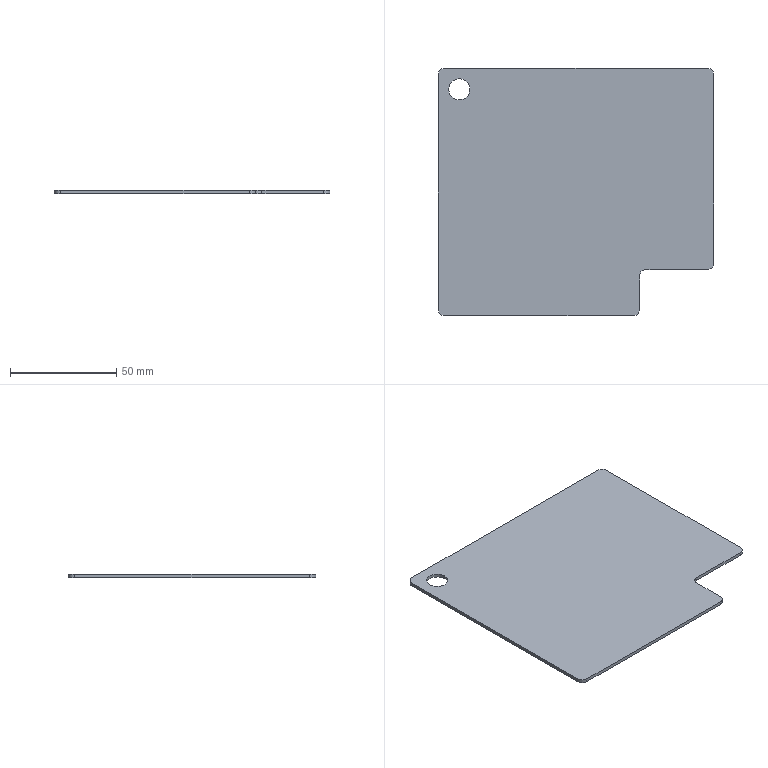Part | SolidWorks | features FlatPattern 1, SMBaseFlange 1, SheetMetal 1 | 1 solid | 16 faces | box 130 x 116.815 x 1.6 mm | volume 22938 mm3 | cylinder 8 | plane 8 | commonest cylinder face diameters 6 x6 10 x2
STEP:
#1=CARTESIAN_POINT('',(5.,272.5,1.6));
#2=VERTEX_POINT('',#1);
#3=CARTESIAN_POINT('',(15.,272.5,1.6));
#4=VERTEX_POINT('',#3);
#5=CARTESIAN_POINT('',(10.,272.5,1.6));
#6=DIRECTION('',(0.,0.,1.));
#7=DIRECTION('',(1.,0.,0.));
#8=AXIS2_PLACEMENT_3D('',#5,#6,#7);
#9=CIRCLE('',#8,5.);
#10=EDGE_CURVE('',#2,#4,#9,.T.);
#11=ORIENTED_EDGE('',*,*,#10,.T.);
#12=CARTESIAN_POINT('',(15.,272.5,0.));
#13=VERTEX_POINT('',#12);
#14=CARTESIAN_POINT('',(15.,272.5,1.6));
#15=DIRECTION('',(0.,0.,-1.));
#16=VECTOR('',#15,1000.);
#17=LINE('',#14,#16);
#18=EDGE_CURVE('',#4,#13,#17,.T.);
#19=ORIENTED_EDGE('',*,*,#18,.T.);
#20=CARTESIAN_POINT('',(5.,272.5,0.));
#21=VERTEX_POINT('',#20);
#22=CARTESIAN_POINT('',(10.,272.5,0.));
#23=DIRECTION('',(0.,0.,1.));
#24=DIRECTION('',(1.,0.,0.));
#25=AXIS2_PLACEMENT_3D('',#22,#23,#24);
#26=CIRCLE('',#25,5.);
#27=EDGE_CURVE('',#21,#13,#26,.T.);
#28=ORIENTED_EDGE('',*,*,#27,.F.);
#29=CARTESIAN_POINT('',(5.,272.5,1.6));
#30=DIRECTION('',(0.,0.,-1.));
#31=VECTOR('',#30,1000.);
#32=LINE('',#29,#31);
#33=EDGE_CURVE('',#2,#21,#32,.T.);
#34=ORIENTED_EDGE('',*,*,#33,.F.);
#35=EDGE_LOOP('',(#11,#19,#28,#34));
#36=FACE_OUTER_BOUND('',#35,.T.);
#37=CARTESIAN_POINT('',(10.,272.5,1.6));
#38=DIRECTION('',(0.,0.,-1.));
#39=DIRECTION('',(-1.,0.,0.));
#40=AXIS2_PLACEMENT_3D('',#37,#38,#39);
#41=CYLINDRICAL_SURFACE('',#40,5.);
#42=ADVANCED_FACE('',(#36),#41,.F.);
#43=CARTESIAN_POINT('',(0.,168.685,1.6));
#44=VERTEX_POINT('',#43);
#45=CARTESIAN_POINT('',(3.,165.685,1.6));
#46=VERTEX_POINT('',#45);
#47=CARTESIAN_POINT('',(3.,168.685,1.6));
#48=DIRECTION('',(0.,0.,1.));
#49=DIRECTION('',(-1.,0.,0.));
#50=AXIS2_PLACEMENT_3D('',#47,#48,#49);
#51=CIRCLE('',#50,3.);
#52=EDGE_CURVE('',#44,#46,#51,.T.);
#53=ORIENTED_EDGE('',*,*,#52,.T.);
#54=CARTESIAN_POINT('',(92.,165.685,1.6));
#55=VERTEX_POINT('',#54);
#56=CARTESIAN_POINT('',(92.,165.685,1.6));
#57=DIRECTION('',(1.,0.,0.));
#58=VECTOR('',#57,1000.);
#59=LINE('',#56,#58);
#60=EDGE_CURVE('',#46,#55,#59,.T.);
#61=ORIENTED_EDGE('',*,*,#60,.T.);
#62=CARTESIAN_POINT('',(95.,168.685,1.6));
#63=VERTEX_POINT('',#62);
#64=CARTESIAN_POINT('',(92.,168.685,1.6));
#65=DIRECTION('',(0.,0.,1.));
#66=DIRECTION('',(-1.,0.,0.));
#67=AXIS2_PLACEMENT_3D('',#64,#65,#66);
#68=CIRCLE('',#67,3.);
#69=EDGE_CURVE('',#55,#63,#68,.T.);
#70=ORIENTED_EDGE('',*,*,#69,.T.);
#71=CARTESIAN_POINT('',(95.,184.5,1.6));
#72=VERTEX_POINT('',#71);
#73=CARTESIAN_POINT('',(95.,184.5,1.6));
#74=DIRECTION('',(0.,1.,0.));
#75=VECTOR('',#74,1000.);
#76=LINE('',#73,#75);
#77=EDGE_CURVE('',#63,#72,#76,.T.);
#78=ORIENTED_EDGE('',*,*,#77,.T.);
#79=CARTESIAN_POINT('',(98.,187.5,1.6));
#80=VERTEX_POINT('',#79);
#81=CARTESIAN_POINT('',(98.,184.5,1.6));
#82=DIRECTION('',(0.,0.,-1.));
#83=DIRECTION('',(1.,0.,0.));
#84=AXIS2_PLACEMENT_3D('',#81,#82,#83);
#85=CIRCLE('',#84,3.);
#86=EDGE_CURVE('',#72,#80,#85,.T.);
#87=ORIENTED_EDGE('',*,*,#86,.T.);
#88=CARTESIAN_POINT('',(127.,187.5,1.6));
#89=VERTEX_POINT('',#88);
#90=CARTESIAN_POINT('',(127.,187.5,1.6));
#91=DIRECTION('',(1.,0.,0.));
#92=VECTOR('',#91,1000.);
#93=LINE('',#90,#92);
#94=EDGE_CURVE('',#80,#89,#93,.T.);
#95=ORIENTED_EDGE('',*,*,#94,.T.);
#96=CARTESIAN_POINT('',(130.,190.5,1.6));
#97=VERTEX_POINT('',#96);
#98=CARTESIAN_POINT('',(127.,190.5,1.6));
#99=DIRECTION('',(0.,0.,1.));
#100=DIRECTION('',(-1.,0.,0.));
#101=AXIS2_PLACEMENT_3D('',#98,#99,#100);
#102=CIRCLE('',#101,3.);
#103=EDGE_CURVE('',#89,#97,#102,.T.);
#104=ORIENTED_EDGE('',*,*,#103,.T.);
#105=CARTESIAN_POINT('',(130.,279.5,1.6));
#106=VERTEX_POINT('',#105);
#107=CARTESIAN_POINT('',(130.,279.5,1.6));
#108=DIRECTION('',(0.,1.,0.));
#109=VECTOR('',#108,1000.);
#110=LINE('',#107,#109);
#111=EDGE_CURVE('',#97,#106,#110,.T.);
#112=ORIENTED_EDGE('',*,*,#111,.T.);
#113=CARTESIAN_POINT('',(127.,282.5,1.6));
#114=VERTEX_POINT('',#113);
#115=CARTESIAN_POINT('',(127.,279.5,1.6));
#116=DIRECTION('',(0.,0.,1.));
#117=DIRECTION('',(-1.,0.,0.));
#118=AXIS2_PLACEMENT_3D('',#115,#116,#117);
#119=CIRCLE('',#118,3.);
#120=EDGE_CURVE('',#106,#114,#119,.T.);
#121=ORIENTED_EDGE('',*,*,#120,.T.);
#122=CARTESIAN_POINT('',(3.,282.5,1.6));
#123=VERTEX_POINT('',#122);
#124=CARTESIAN_POINT('',(3.,282.5,1.6));
#125=DIRECTION('',(-1.,0.,0.));
#126=VECTOR('',#125,1000.);
#127=LINE('',#124,#126);
#128=EDGE_CURVE('',#114,#123,#127,.T.);
#129=ORIENTED_EDGE('',*,*,#128,.T.);
#130=CARTESIAN_POINT('',(0.,279.5,1.6));
#131=VERTEX_POINT('',#130);
#132=CARTESIAN_POINT('',(3.,279.5,1.6));
#133=DIRECTION('',(0.,0.,1.));
#134=DIRECTION('',(1.,0.,0.));
#135=AXIS2_PLACEMENT_3D('',#132,#133,#134);
#136=CIRCLE('',#135,3.);
#137=EDGE_CURVE('',#123,#131,#136,.T.);
#138=ORIENTED_EDGE('',*,*,#137,.T.);
#139=CARTESIAN_POINT('',(0.,168.685,1.6));
#140=DIRECTION('',(0.,-1.,0.));
#141=VECTOR('',#140,1000.);
#142=LINE('',#139,#141);
#143=EDGE_CURVE('',#131,#44,#142,.T.);
#144=ORIENTED_EDGE('',*,*,#143,.T.);
#145=EDGE_LOOP('',(#53,#61,#70,#78,#87,#95,#104,#112,#121,#129,#138,#144));
#146=FACE_OUTER_BOUND('',#145,.T.);
#147=ORIENTED_EDGE('',*,*,#10,.F.);
#148=CARTESIAN_POINT('',(10.,272.5,1.6));
#149=DIRECTION('',(0.,0.,1.));
#150=DIRECTION('',(1.,0.,0.));
#151=AXIS2_PLACEMENT_3D('',#148,#149,#150);
#152=CIRCLE('',#151,5.);
#153=EDGE_CURVE('',#4,#2,#152,.T.);
#154=ORIENTED_EDGE('',*,*,#153,.F.);
#155=EDGE_LOOP('',(#147,#154));
#156=FACE_BOUND('',#155,.T.);
#157=CARTESIAN_POINT('',(3.,168.685,1.6));
#158=DIRECTION('',(0.,0.,-1.));
#159=DIRECTION('',(-1.,0.,0.));
#160=AXIS2_PLACEMENT_3D('',#157,#158,#159);
#161=PLANE('',#160);
#162=ADVANCED_FACE('',(#146,#156),#161,.F.);
#163=CARTESIAN_POINT('',(0.,168.685,0.));
#164=VERTEX_POINT('',#163);
#165=CARTESIAN_POINT('',(3.,165.685,0.));
#166=VERTEX_POINT('',#165);
#167=CARTESIAN_POINT('',(3.,168.685,0.));
#168=DIRECTION('',(0.,0.,1.));
#169=DIRECTION('',(-1.,0.,0.));
#170=AXIS2_PLACEMENT_3D('',#167,#168,#169);
#171=CIRCLE('',#170,3.);
#172=EDGE_CURVE('',#164,#166,#171,.T.);
#173=ORIENTED_EDGE('',*,*,#172,.F.);
#174=CARTESIAN_POINT('',(0.,279.5,0.));
#175=VERTEX_POINT('',#174);
#176=CARTESIAN_POINT('',(0.,168.685,0.));
#177=DIRECTION('',(0.,-1.,0.));
#178=VECTOR('',#177,1000.);
#179=LINE('',#176,#178);
#180=EDGE_CURVE('',#175,#164,#179,.T.);
#181=ORIENTED_EDGE('',*,*,#180,.F.);
#182=CARTESIAN_POINT('',(3.,282.5,0.));
#183=VERTEX_POINT('',#182);
#184=CARTESIAN_POINT('',(3.,279.5,0.));
#185=DIRECTION('',(0.,0.,1.));
#186=DIRECTION('',(1.,0.,0.));
#187=AXIS2_PLACEMENT_3D('',#184,#185,#186);
#188=CIRCLE('',#187,3.);
#189=EDGE_CURVE('',#183,#175,#188,.T.);
#190=ORIENTED_EDGE('',*,*,#189,.F.);
#191=CARTESIAN_POINT('',(127.,282.5,0.));
#192=VERTEX_POINT('',#191);
#193=CARTESIAN_POINT('',(3.,282.5,0.));
#194=DIRECTION('',(-1.,0.,0.));
#195=VECTOR('',#194,1000.);
#196=LINE('',#193,#195);
#197=EDGE_CURVE('',#192,#183,#196,.T.);
#198=ORIENTED_EDGE('',*,*,#197,.F.);
#199=CARTESIAN_POINT('',(130.,279.5,0.));
#200=VERTEX_POINT('',#199);
#201=CARTESIAN_POINT('',(127.,279.5,0.));
#202=DIRECTION('',(0.,0.,1.));
#203=DIRECTION('',(-1.,0.,0.));
#204=AXIS2_PLACEMENT_3D('',#201,#202,#203);
#205=CIRCLE('',#204,3.);
#206=EDGE_CURVE('',#200,#192,#205,.T.);
#207=ORIENTED_EDGE('',*,*,#206,.F.);
#208=CARTESIAN_POINT('',(130.,190.5,0.));
#209=VERTEX_POINT('',#208);
#210=CARTESIAN_POINT('',(130.,279.5,0.));
#211=DIRECTION('',(0.,1.,0.));
#212=VECTOR('',#211,1000.);
#213=LINE('',#210,#212);
#214=EDGE_CURVE('',#209,#200,#213,.T.);
#215=ORIENTED_EDGE('',*,*,#214,.F.);
#216=CARTESIAN_POINT('',(127.,187.5,0.));
#217=VERTEX_POINT('',#216);
#218=CARTESIAN_POINT('',(127.,190.5,0.));
#219=DIRECTION('',(0.,0.,1.));
#220=DIRECTION('',(-1.,0.,0.));
#221=AXIS2_PLACEMENT_3D('',#218,#219,#220);
#222=CIRCLE('',#221,3.);
#223=EDGE_CURVE('',#217,#209,#222,.T.);
#224=ORIENTED_EDGE('',*,*,#223,.F.);
#225=CARTESIAN_POINT('',(98.,187.5,0.));
#226=VERTEX_POINT('',#225);
#227=CARTESIAN_POINT('',(127.,187.5,0.));
#228=DIRECTION('',(1.,0.,0.));
#229=VECTOR('',#228,1000.);
#230=LINE('',#227,#229);
#231=EDGE_CURVE('',#226,#217,#230,.T.);
#232=ORIENTED_EDGE('',*,*,#231,.F.);
#233=CARTESIAN_POINT('',(95.,184.5,0.));
#234=VERTEX_POINT('',#233);
#235=CARTESIAN_POINT('',(98.,184.5,0.));
#236=DIRECTION('',(0.,0.,-1.));
#237=DIRECTION('',(1.,0.,0.));
#238=AXIS2_PLACEMENT_3D('',#235,#236,#237);
#239=CIRCLE('',#238,3.);
#240=EDGE_CURVE('',#234,#226,#239,.T.);
#241=ORIENTED_EDGE('',*,*,#240,.F.);
#242=CARTESIAN_POINT('',(95.,168.685,0.));
#243=VERTEX_POINT('',#242);
#244=CARTESIAN_POINT('',(95.,184.5,0.));
#245=DIRECTION('',(0.,1.,0.));
#246=VECTOR('',#245,1000.);
#247=LINE('',#244,#246);
#248=EDGE_CURVE('',#243,#234,#247,.T.);
#249=ORIENTED_EDGE('',*,*,#248,.F.);
#250=CARTESIAN_POINT('',(92.,165.685,0.));
#251=VERTEX_POINT('',#250);
#252=CARTESIAN_POINT('',(92.,168.685,0.));
#253=DIRECTION('',(0.,0.,1.));
#254=DIRECTION('',(-1.,0.,0.));
#255=AXIS2_PLACEMENT_3D('',#252,#253,#254);
#256=CIRCLE('',#255,3.);
#257=EDGE_CURVE('',#251,#243,#256,.T.);
#258=ORIENTED_EDGE('',*,*,#257,.F.);
#259=CARTESIAN_POINT('',(92.,165.685,0.));
#260=DIRECTION('',(1.,0.,0.));
#261=VECTOR('',#260,1000.);
#262=LINE('',#259,#261);
#263=EDGE_CURVE('',#166,#251,#262,.T.);
#264=ORIENTED_EDGE('',*,*,#263,.F.);
#265=EDGE_LOOP('',(#173,#181,#190,#198,#207,#215,#224,#232,#241,#249,#258,#264));
#266=FACE_OUTER_BOUND('',#265,.T.);
#267=ORIENTED_EDGE('',*,*,#27,.T.);
#268=CARTESIAN_POINT('',(10.,272.5,0.));
#269=DIRECTION('',(0.,0.,1.));
#270=DIRECTION('',(1.,0.,0.));
#271=AXIS2_PLACEMENT_3D('',#268,#269,#270);
#272=CIRCLE('',#271,5.);
#273=EDGE_CURVE('',#13,#21,#272,.T.);
#274=ORIENTED_EDGE('',*,*,#273,.T.);
#275=EDGE_LOOP('',(#267,#274));
#276=FACE_BOUND('',#275,.T.);
#277=CARTESIAN_POINT('',(3.,168.685,0.));
#278=DIRECTION('',(0.,0.,-1.));
#279=DIRECTION('',(-1.,0.,0.));
#280=AXIS2_PLACEMENT_3D('',#277,#278,#279);
#281=PLANE('',#280);
#282=ADVANCED_FACE('',(#266,#276),#281,.T.);
#283=ORIENTED_EDGE('',*,*,#172,.T.);
#284=CARTESIAN_POINT('',(3.,165.685,1.6));
#285=DIRECTION('',(0.,0.,-1.));
#286=VECTOR('',#285,1000.);
#287=LINE('',#284,#286);
#288=EDGE_CURVE('',#46,#166,#287,.T.);
#289=ORIENTED_EDGE('',*,*,#288,.F.);
#290=ORIENTED_EDGE('',*,*,#52,.F.);
#291=CARTESIAN_POINT('',(0.,168.685,1.6));
#292=DIRECTION('',(0.,0.,-1.));
#293=VECTOR('',#292,1000.);
#294=LINE('',#291,#293);
#295=EDGE_CURVE('',#44,#164,#294,.T.);
#296=ORIENTED_EDGE('',*,*,#295,.T.);
#297=EDGE_LOOP('',(#283,#289,#290,#296));
#298=FACE_OUTER_BOUND('',#297,.T.);
#299=CARTESIAN_POINT('',(3.,168.685,1.6));
#300=DIRECTION('',(0.,0.,-1.));
#301=DIRECTION('',(-1.,0.,0.));
#302=AXIS2_PLACEMENT_3D('',#299,#300,#301);
#303=CYLINDRICAL_SURFACE('',#302,3.);
#304=ADVANCED_FACE('',(#298),#303,.T.);
#305=ORIENTED_EDGE('',*,*,#263,.T.);
#306=CARTESIAN_POINT('',(92.,165.685,1.6));
#307=DIRECTION('',(0.,0.,-1.));
#308=VECTOR('',#307,1000.);
#309=LINE('',#306,#308);
#310=EDGE_CURVE('',#55,#251,#309,.T.);
#311=ORIENTED_EDGE('',*,*,#310,.F.);
#312=ORIENTED_EDGE('',*,*,#60,.F.);
#313=ORIENTED_EDGE('',*,*,#288,.T.);
#314=EDGE_LOOP('',(#305,#311,#312,#313));
#315=FACE_OUTER_BOUND('',#314,.T.);
#316=CARTESIAN_POINT('',(92.,165.685,1.6));
#317=DIRECTION('',(0.,1.,0.));
#318=DIRECTION('',(0.,0.,1.));
#319=AXIS2_PLACEMENT_3D('',#316,#317,#318);
#320=PLANE('',#319);
#321=ADVANCED_FACE('',(#315),#320,.F.);
#322=ORIENTED_EDGE('',*,*,#257,.T.);
#323=CARTESIAN_POINT('',(95.,168.685,1.6));
#324=DIRECTION('',(0.,0.,-1.));
#325=VECTOR('',#324,1000.);
#326=LINE('',#323,#325);
#327=EDGE_CURVE('',#63,#243,#326,.T.);
#328=ORIENTED_EDGE('',*,*,#327,.F.);
#329=ORIENTED_EDGE('',*,*,#69,.F.);
#330=ORIENTED_EDGE('',*,*,#310,.T.);
#331=EDGE_LOOP('',(#322,#328,#329,#330));
#332=FACE_OUTER_BOUND('',#331,.T.);
#333=CARTESIAN_POINT('',(92.,168.685,1.6));
#334=DIRECTION('',(0.,0.,-1.));
#335=DIRECTION('',(-1.,0.,0.));
#336=AXIS2_PLACEMENT_3D('',#333,#334,#335);
#337=CYLINDRICAL_SURFACE('',#336,3.);
#338=ADVANCED_FACE('',(#332),#337,.T.);
#339=ORIENTED_EDGE('',*,*,#248,.T.);
#340=CARTESIAN_POINT('',(95.,184.5,1.6));
#341=DIRECTION('',(0.,0.,-1.));
#342=VECTOR('',#341,1000.);
#343=LINE('',#340,#342);
#344=EDGE_CURVE('',#72,#234,#343,.T.);
#345=ORIENTED_EDGE('',*,*,#344,.F.);
#346=ORIENTED_EDGE('',*,*,#77,.F.);
#347=ORIENTED_EDGE('',*,*,#327,.T.);
#348=EDGE_LOOP('',(#339,#345,#346,#347));
#349=FACE_OUTER_BOUND('',#348,.T.);
#350=CARTESIAN_POINT('',(95.,184.5,1.6));
#351=DIRECTION('',(-1.,0.,0.));
#352=DIRECTION('',(0.,0.,1.));
#353=AXIS2_PLACEMENT_3D('',#350,#351,#352);
#354=PLANE('',#353);
#355=ADVANCED_FACE('',(#349),#354,.F.);
#356=ORIENTED_EDGE('',*,*,#240,.T.);
#357=CARTESIAN_POINT('',(98.,187.5,1.6));
#358=DIRECTION('',(0.,0.,-1.));
#359=VECTOR('',#358,1000.);
#360=LINE('',#357,#359);
#361=EDGE_CURVE('',#80,#226,#360,.T.);
#362=ORIENTED_EDGE('',*,*,#361,.F.);
#363=ORIENTED_EDGE('',*,*,#86,.F.);
#364=ORIENTED_EDGE('',*,*,#344,.T.);
#365=EDGE_LOOP('',(#356,#362,#363,#364));
#366=FACE_OUTER_BOUND('',#365,.T.);
#367=CARTESIAN_POINT('',(98.,184.5,1.6));
#368=DIRECTION('',(0.,0.,-1.));
#369=DIRECTION('',(-1.,0.,0.));
#370=AXIS2_PLACEMENT_3D('',#367,#368,#369);
#371=CYLINDRICAL_SURFACE('',#370,3.);
#372=ADVANCED_FACE('',(#366),#371,.F.);
#373=ORIENTED_EDGE('',*,*,#231,.T.);
#374=CARTESIAN_POINT('',(127.,187.5,1.6));
#375=DIRECTION('',(0.,0.,-1.));
#376=VECTOR('',#375,1000.);
#377=LINE('',#374,#376);
#378=EDGE_CURVE('',#89,#217,#377,.T.);
#379=ORIENTED_EDGE('',*,*,#378,.F.);
#380=ORIENTED_EDGE('',*,*,#94,.F.);
#381=ORIENTED_EDGE('',*,*,#361,.T.);
#382=EDGE_LOOP('',(#373,#379,#380,#381));
#383=FACE_OUTER_BOUND('',#382,.T.);
#384=CARTESIAN_POINT('',(127.,187.5,1.6));
#385=DIRECTION('',(0.,1.,0.));
#386=DIRECTION('',(-1.,0.,0.));
#387=AXIS2_PLACEMENT_3D('',#384,#385,#386);
#388=PLANE('',#387);
#389=ADVANCED_FACE('',(#383),#388,.F.);
#390=ORIENTED_EDGE('',*,*,#223,.T.);
#391=CARTESIAN_POINT('',(130.,190.5,1.6));
#392=DIRECTION('',(0.,0.,-1.));
#393=VECTOR('',#392,1000.);
#394=LINE('',#391,#393);
#395=EDGE_CURVE('',#97,#209,#394,.T.);
#396=ORIENTED_EDGE('',*,*,#395,.F.);
#397=ORIENTED_EDGE('',*,*,#103,.F.);
#398=ORIENTED_EDGE('',*,*,#378,.T.);
#399=EDGE_LOOP('',(#390,#396,#397,#398));
#400=FACE_OUTER_BOUND('',#399,.T.);
#401=CARTESIAN_POINT('',(127.,190.5,1.6));
#402=DIRECTION('',(0.,0.,-1.));
#403=DIRECTION('',(-1.,0.,0.));
#404=AXIS2_PLACEMENT_3D('',#401,#402,#403);
#405=CYLINDRICAL_SURFACE('',#404,3.);
#406=ADVANCED_FACE('',(#400),#405,.T.);
#407=ORIENTED_EDGE('',*,*,#214,.T.);
#408=CARTESIAN_POINT('',(130.,279.5,1.6));
#409=DIRECTION('',(0.,0.,-1.));
#410=VECTOR('',#409,1000.);
#411=LINE('',#408,#410);
#412=EDGE_CURVE('',#106,#200,#411,.T.);
#413=ORIENTED_EDGE('',*,*,#412,.F.);
#414=ORIENTED_EDGE('',*,*,#111,.F.);
#415=ORIENTED_EDGE('',*,*,#395,.T.);
#416=EDGE_LOOP('',(#407,#413,#414,#415));
#417=FACE_OUTER_BOUND('',#416,.T.);
#418=CARTESIAN_POINT('',(130.,279.5,1.6));
#419=DIRECTION('',(-1.,0.,0.));
#420=DIRECTION('',(0.,0.,1.));
#421=AXIS2_PLACEMENT_3D('',#418,#419,#420);
#422=PLANE('',#421);
#423=ADVANCED_FACE('',(#417),#422,.F.);
#424=ORIENTED_EDGE('',*,*,#206,.T.);
#425=CARTESIAN_POINT('',(127.,282.5,1.6));
#426=DIRECTION('',(0.,0.,-1.));
#427=VECTOR('',#426,1000.);
#428=LINE('',#425,#427);
#429=EDGE_CURVE('',#114,#192,#428,.T.);
#430=ORIENTED_EDGE('',*,*,#429,.F.);
#431=ORIENTED_EDGE('',*,*,#120,.F.);
#432=ORIENTED_EDGE('',*,*,#412,.T.);
#433=EDGE_LOOP('',(#424,#430,#431,#432));
#434=FACE_OUTER_BOUND('',#433,.T.);
#435=CARTESIAN_POINT('',(127.,279.5,1.6));
#436=DIRECTION('',(0.,0.,-1.));
#437=DIRECTION('',(-1.,0.,0.));
#438=AXIS2_PLACEMENT_3D('',#435,#436,#437);
#439=CYLINDRICAL_SURFACE('',#438,3.);
#440=ADVANCED_FACE('',(#434),#439,.T.);
#441=ORIENTED_EDGE('',*,*,#197,.T.);
#442=CARTESIAN_POINT('',(3.,282.5,1.6));
#443=DIRECTION('',(0.,0.,-1.));
#444=VECTOR('',#443,1000.);
#445=LINE('',#442,#444);
#446=EDGE_CURVE('',#123,#183,#445,.T.);
#447=ORIENTED_EDGE('',*,*,#446,.F.);
#448=ORIENTED_EDGE('',*,*,#128,.F.);
#449=ORIENTED_EDGE('',*,*,#429,.T.);
#450=EDGE_LOOP('',(#441,#447,#448,#449));
#451=FACE_OUTER_BOUND('',#450,.T.);
#452=CARTESIAN_POINT('',(3.,282.5,1.6));
#453=DIRECTION('',(0.,-1.,0.));
#454=DIRECTION('',(0.,0.,-1.));
#455=AXIS2_PLACEMENT_3D('',#452,#453,#454);
#456=PLANE('',#455);
#457=ADVANCED_FACE('',(#451),#456,.F.);
#458=ORIENTED_EDGE('',*,*,#189,.T.);
#459=CARTESIAN_POINT('',(0.,279.5,1.6));
#460=DIRECTION('',(0.,0.,-1.));
#461=VECTOR('',#460,1000.);
#462=LINE('',#459,#461);
#463=EDGE_CURVE('',#131,#175,#462,.T.);
#464=ORIENTED_EDGE('',*,*,#463,.F.);
#465=ORIENTED_EDGE('',*,*,#137,.F.);
#466=ORIENTED_EDGE('',*,*,#446,.T.);
#467=EDGE_LOOP('',(#458,#464,#465,#466));
#468=FACE_OUTER_BOUND('',#467,.T.);
#469=CARTESIAN_POINT('',(3.,279.5,1.6));
#470=DIRECTION('',(0.,0.,-1.));
#471=DIRECTION('',(-1.,0.,0.));
#472=AXIS2_PLACEMENT_3D('',#469,#470,#471);
#473=CYLINDRICAL_SURFACE('',#472,3.);
#474=ADVANCED_FACE('',(#468),#473,.T.);
#475=ORIENTED_EDGE('',*,*,#180,.T.);
#476=ORIENTED_EDGE('',*,*,#295,.F.);
#477=ORIENTED_EDGE('',*,*,#143,.F.);
#478=ORIENTED_EDGE('',*,*,#463,.T.);
#479=EDGE_LOOP('',(#475,#476,#477,#478));
#480=FACE_OUTER_BOUND('',#479,.T.);
#481=CARTESIAN_POINT('',(0.,168.685,1.6));
#482=DIRECTION('',(1.,0.,0.));
#483=DIRECTION('',(0.,1.,0.));
#484=AXIS2_PLACEMENT_3D('',#481,#482,#483);
#485=PLANE('',#484);
#486=ADVANCED_FACE('',(#480),#485,.F.);
#487=ORIENTED_EDGE('',*,*,#18,.F.);
#488=ORIENTED_EDGE('',*,*,#153,.T.);
#489=ORIENTED_EDGE('',*,*,#33,.T.);
#490=ORIENTED_EDGE('',*,*,#273,.F.);
#491=EDGE_LOOP('',(#487,#488,#489,#490));
#492=FACE_OUTER_BOUND('',#491,.T.);
#493=CARTESIAN_POINT('',(10.,272.5,1.6));
#494=DIRECTION('',(0.,0.,-1.));
#495=DIRECTION('',(-1.,0.,0.));
#496=AXIS2_PLACEMENT_3D('',#493,#494,#495);
#497=CYLINDRICAL_SURFACE('',#496,5.);
#498=ADVANCED_FACE('',(#492),#497,.F.);
#499=CLOSED_SHELL('',(#42,#162,#282,#304,#321,#338,#355,#372,#389,#406,#423,#440,#457,#474,#486,#498));
#500=MANIFOLD_SOLID_BREP('',#499);
#501=CARTESIAN_POINT('',(0.,0.,0.));
#502=DIRECTION('',(0.,0.,1.));
#503=DIRECTION('',(1.,0.,0.));
#504=AXIS2_PLACEMENT_3D('',#501,#502,#503);
#505=(LENGTH_UNIT()NAMED_UNIT(*)SI_UNIT(.MILLI.,.METRE.));
#506=UNCERTAINTY_MEASURE_WITH_UNIT(LENGTH_MEASURE(0.00001),#505,'','');
#507=(NAMED_UNIT(*)PLANE_ANGLE_UNIT()SI_UNIT($,.RADIAN.));
#508=(NAMED_UNIT(*)SI_UNIT($,.STERADIAN.)SOLID_ANGLE_UNIT());
#509=(GEOMETRIC_REPRESENTATION_CONTEXT(3)GLOBAL_UNCERTAINTY_ASSIGNED_CONTEXT((#506))GLOBAL_UNIT_ASSIGNED_CONTEXT((#505,#507,#508))REPRESENTATION_CONTEXT('',''));
#510=ADVANCED_BREP_SHAPE_REPRESENTATION('',(#500,#504),#509);